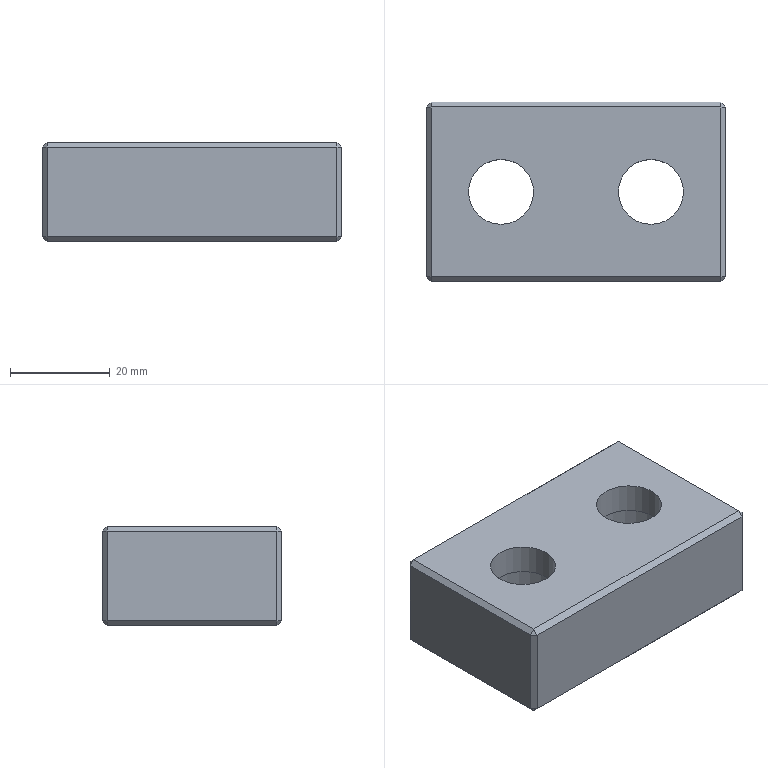Part | NX | features solid 2 | 1 solid | 32 faces | box 60 x 36 x 20 mm | volume 32584 mm3 | plane 28 | cylinder 4 | commonest cylinder face diameters 13 x2 20 x2
STEP:
#1=CARTESIAN_POINT('',(-28.,-137.,200.));
#2=VERTEX_POINT('',#1);
#3=CARTESIAN_POINT('',(30.,-137.,200.));
#4=VERTEX_POINT('',#3);
#5=CARTESIAN_POINT('',(-29.,-137.,200.));
#6=DIRECTION('',(-1.,0.,0.));
#7=VECTOR('',#6,1000.);
#8=LINE('',#5,#7);
#9=EDGE_CURVE('',#2,#4,#8,.F.);
#10=ORIENTED_EDGE('',*,*,#9,.F.);
#11=CARTESIAN_POINT('',(-28.,-171.,200.));
#12=VERTEX_POINT('',#11);
#13=CARTESIAN_POINT('',(-28.,-178.,200.));
#14=DIRECTION('',(0.,-1.,0.));
#15=VECTOR('',#14,1000.);
#16=LINE('',#13,#15);
#17=EDGE_CURVE('',#12,#2,#16,.F.);
#18=ORIENTED_EDGE('',*,*,#17,.F.);
#19=CARTESIAN_POINT('',(30.,-171.,200.));
#20=VERTEX_POINT('',#19);
#21=CARTESIAN_POINT('',(-29.,-171.,200.));
#22=DIRECTION('',(1.,0.,0.));
#23=VECTOR('',#22,1000.);
#24=LINE('',#21,#23);
#25=EDGE_CURVE('',#20,#12,#24,.F.);
#26=ORIENTED_EDGE('',*,*,#25,.F.);
#27=CARTESIAN_POINT('',(30.,-178.,200.));
#28=DIRECTION('',(0.,1.,0.));
#29=VECTOR('',#28,1000.);
#30=LINE('',#27,#29);
#31=EDGE_CURVE('',#4,#20,#30,.F.);
#32=ORIENTED_EDGE('',*,*,#31,.F.);
#33=EDGE_LOOP('',(#10,#18,#26,#32));
#34=FACE_BOUND('',#33,.T.);
#35=CARTESIAN_POINT('',(-14.,-147.5,200.));
#36=VERTEX_POINT('',#35);
#37=CARTESIAN_POINT('',(-14.,-154.,200.));
#38=DIRECTION('',(0.,0.,1.));
#39=DIRECTION('',(0.,1.,0.));
#40=AXIS2_PLACEMENT_3D('',#37,#38,#39);
#41=CIRCLE('',#40,6.5);
#42=EDGE_CURVE('',#36,#36,#41,.T.);
#43=ORIENTED_EDGE('',*,*,#42,.F.);
#44=EDGE_LOOP('',(#43));
#45=FACE_BOUND('',#44,.T.);
#46=CARTESIAN_POINT('',(16.,-147.5,200.));
#47=VERTEX_POINT('',#46);
#48=CARTESIAN_POINT('',(16.,-154.,200.));
#49=DIRECTION('',(0.,0.,1.));
#50=DIRECTION('',(0.,1.,0.));
#51=AXIS2_PLACEMENT_3D('',#48,#49,#50);
#52=CIRCLE('',#51,6.5);
#53=EDGE_CURVE('',#47,#47,#52,.T.);
#54=ORIENTED_EDGE('',*,*,#53,.F.);
#55=EDGE_LOOP('',(#54));
#56=FACE_BOUND('',#55,.T.);
#57=CARTESIAN_POINT('',(-29.,-178.,200.));
#58=DIRECTION('',(0.,0.,-1.));
#59=DIRECTION('',(1.,0.,0.));
#60=AXIS2_PLACEMENT_3D('',#57,#58,#59);
#61=PLANE('',#60);
#62=ADVANCED_FACE('',(#34,#45,#56),#61,.F.);
#63=CARTESIAN_POINT('',(16.,-144.,194.));
#64=VERTEX_POINT('',#63);
#65=CARTESIAN_POINT('',(16.,-154.,194.));
#66=DIRECTION('',(0.,0.,1.));
#67=DIRECTION('',(0.,1.,0.));
#68=AXIS2_PLACEMENT_3D('',#65,#66,#67);
#69=CIRCLE('',#68,10.);
#70=EDGE_CURVE('',#64,#64,#69,.T.);
#71=ORIENTED_EDGE('',*,*,#70,.F.);
#72=EDGE_LOOP('',(#71));
#73=FACE_BOUND('',#72,.T.);
#74=CARTESIAN_POINT('',(16.,-147.5,194.));
#75=VERTEX_POINT('',#74);
#76=CARTESIAN_POINT('',(16.,-154.,194.));
#77=DIRECTION('',(0.,0.,1.));
#78=DIRECTION('',(0.,1.,0.));
#79=AXIS2_PLACEMENT_3D('',#76,#77,#78);
#80=CIRCLE('',#79,6.5);
#81=EDGE_CURVE('',#75,#75,#80,.F.);
#82=ORIENTED_EDGE('',*,*,#81,.F.);
#83=EDGE_LOOP('',(#82));
#84=FACE_BOUND('',#83,.T.);
#85=CARTESIAN_POINT('',(16.,-154.,194.));
#86=DIRECTION('',(0.,0.,-1.));
#87=DIRECTION('',(0.,1.,0.));
#88=AXIS2_PLACEMENT_3D('',#85,#86,#87);
#89=PLANE('',#88);
#90=ADVANCED_FACE('',(#73,#84),#89,.T.);
#91=CARTESIAN_POINT('',(-14.,-144.,194.));
#92=VERTEX_POINT('',#91);
#93=CARTESIAN_POINT('',(-14.,-154.,194.));
#94=DIRECTION('',(0.,0.,1.));
#95=DIRECTION('',(0.,1.,0.));
#96=AXIS2_PLACEMENT_3D('',#93,#94,#95);
#97=CIRCLE('',#96,10.);
#98=EDGE_CURVE('',#92,#92,#97,.T.);
#99=ORIENTED_EDGE('',*,*,#98,.F.);
#100=EDGE_LOOP('',(#99));
#101=FACE_BOUND('',#100,.T.);
#102=CARTESIAN_POINT('',(-14.,-147.5,194.));
#103=VERTEX_POINT('',#102);
#104=CARTESIAN_POINT('',(-14.,-154.,194.));
#105=DIRECTION('',(0.,0.,1.));
#106=DIRECTION('',(0.,1.,0.));
#107=AXIS2_PLACEMENT_3D('',#104,#105,#106);
#108=CIRCLE('',#107,6.5);
#109=EDGE_CURVE('',#103,#103,#108,.F.);
#110=ORIENTED_EDGE('',*,*,#109,.F.);
#111=EDGE_LOOP('',(#110));
#112=FACE_BOUND('',#111,.T.);
#113=CARTESIAN_POINT('',(-14.,-154.,194.));
#114=DIRECTION('',(0.,0.,-1.));
#115=DIRECTION('',(0.,1.,0.));
#116=AXIS2_PLACEMENT_3D('',#113,#114,#115);
#117=PLANE('',#116);
#118=ADVANCED_FACE('',(#101,#112),#117,.T.);
#119=CARTESIAN_POINT('',(-28.,-171.,180.));
#120=VERTEX_POINT('',#119);
#121=CARTESIAN_POINT('',(30.,-171.,180.));
#122=VERTEX_POINT('',#121);
#123=CARTESIAN_POINT('',(31.,-171.,180.));
#124=DIRECTION('',(1.,0.,0.));
#125=VECTOR('',#124,1000.);
#126=LINE('',#123,#125);
#127=EDGE_CURVE('',#120,#122,#126,.T.);
#128=ORIENTED_EDGE('',*,*,#127,.F.);
#129=CARTESIAN_POINT('',(-28.,-137.,180.));
#130=VERTEX_POINT('',#129);
#131=CARTESIAN_POINT('',(-28.,-178.,180.));
#132=DIRECTION('',(0.,-1.,0.));
#133=VECTOR('',#132,1000.);
#134=LINE('',#131,#133);
#135=EDGE_CURVE('',#130,#120,#134,.T.);
#136=ORIENTED_EDGE('',*,*,#135,.F.);
#137=CARTESIAN_POINT('',(30.,-137.,180.));
#138=VERTEX_POINT('',#137);
#139=CARTESIAN_POINT('',(-29.,-137.,180.));
#140=DIRECTION('',(-1.,0.,0.));
#141=VECTOR('',#140,1000.);
#142=LINE('',#139,#141);
#143=EDGE_CURVE('',#138,#130,#142,.T.);
#144=ORIENTED_EDGE('',*,*,#143,.F.);
#145=CARTESIAN_POINT('',(30.,-178.,180.));
#146=DIRECTION('',(0.,1.,0.));
#147=VECTOR('',#146,1000.);
#148=LINE('',#145,#147);
#149=EDGE_CURVE('',#122,#138,#148,.T.);
#150=ORIENTED_EDGE('',*,*,#149,.F.);
#151=EDGE_LOOP('',(#128,#136,#144,#150));
#152=FACE_BOUND('',#151,.T.);
#153=CARTESIAN_POINT('',(-14.,-144.,180.));
#154=VERTEX_POINT('',#153);
#155=CARTESIAN_POINT('',(-14.,-154.,180.));
#156=DIRECTION('',(0.,0.,1.));
#157=DIRECTION('',(0.,1.,0.));
#158=AXIS2_PLACEMENT_3D('',#155,#156,#157);
#159=CIRCLE('',#158,10.);
#160=EDGE_CURVE('',#154,#154,#159,.T.);
#161=ORIENTED_EDGE('',*,*,#160,.T.);
#162=EDGE_LOOP('',(#161));
#163=FACE_BOUND('',#162,.T.);
#164=CARTESIAN_POINT('',(16.,-144.,180.));
#165=VERTEX_POINT('',#164);
#166=CARTESIAN_POINT('',(16.,-154.,180.));
#167=DIRECTION('',(0.,0.,1.));
#168=DIRECTION('',(0.,1.,0.));
#169=AXIS2_PLACEMENT_3D('',#166,#167,#168);
#170=CIRCLE('',#169,10.);
#171=EDGE_CURVE('',#165,#165,#170,.T.);
#172=ORIENTED_EDGE('',*,*,#171,.T.);
#173=EDGE_LOOP('',(#172));
#174=FACE_BOUND('',#173,.T.);
#175=CARTESIAN_POINT('',(-29.,-178.,180.));
#176=DIRECTION('',(0.,0.,-1.));
#177=DIRECTION('',(1.,0.,0.));
#178=AXIS2_PLACEMENT_3D('',#175,#176,#177);
#179=PLANE('',#178);
#180=ADVANCED_FACE('',(#152,#163,#174),#179,.T.);
#181=CARTESIAN_POINT('',(-29.,-171.,181.));
#182=VERTEX_POINT('',#181);
#183=CARTESIAN_POINT('',(-29.,-137.,181.));
#184=VERTEX_POINT('',#183);
#185=CARTESIAN_POINT('',(-29.,-178.,181.));
#186=DIRECTION('',(0.,-1.,0.));
#187=VECTOR('',#186,1000.);
#188=LINE('',#185,#187);
#189=EDGE_CURVE('',#182,#184,#188,.F.);
#190=ORIENTED_EDGE('',*,*,#189,.F.);
#191=CARTESIAN_POINT('',(-29.,-171.,199.));
#192=VERTEX_POINT('',#191);
#193=CARTESIAN_POINT('',(-29.,-171.,180.));
#194=DIRECTION('',(0.,0.,1.));
#195=VECTOR('',#194,1000.);
#196=LINE('',#193,#195);
#197=EDGE_CURVE('',#192,#182,#196,.F.);
#198=ORIENTED_EDGE('',*,*,#197,.F.);
#199=CARTESIAN_POINT('',(-29.,-137.,199.));
#200=VERTEX_POINT('',#199);
#201=CARTESIAN_POINT('',(-29.,-178.,199.));
#202=DIRECTION('',(0.,1.,0.));
#203=VECTOR('',#202,1000.);
#204=LINE('',#201,#203);
#205=EDGE_CURVE('',#200,#192,#204,.F.);
#206=ORIENTED_EDGE('',*,*,#205,.F.);
#207=CARTESIAN_POINT('',(-29.,-137.,180.));
#208=DIRECTION('',(0.,0.,-1.));
#209=VECTOR('',#208,1000.);
#210=LINE('',#207,#209);
#211=EDGE_CURVE('',#184,#200,#210,.F.);
#212=ORIENTED_EDGE('',*,*,#211,.F.);
#213=EDGE_LOOP('',(#190,#198,#206,#212));
#214=FACE_BOUND('',#213,.T.);
#215=CARTESIAN_POINT('',(-29.,-178.,180.));
#216=DIRECTION('',(1.,0.,0.));
#217=DIRECTION('',(0.,0.,1.));
#218=AXIS2_PLACEMENT_3D('',#215,#216,#217);
#219=PLANE('',#218);
#220=ADVANCED_FACE('',(#214),#219,.F.);
#221=CARTESIAN_POINT('',(31.,-171.,181.));
#222=VERTEX_POINT('',#221);
#223=CARTESIAN_POINT('',(31.,-171.,199.));
#224=VERTEX_POINT('',#223);
#225=CARTESIAN_POINT('',(31.,-171.,200.));
#226=DIRECTION('',(0.,0.,1.));
#227=VECTOR('',#226,1000.);
#228=LINE('',#225,#227);
#229=EDGE_CURVE('',#222,#224,#228,.T.);
#230=ORIENTED_EDGE('',*,*,#229,.F.);
#231=CARTESIAN_POINT('',(31.,-137.,181.));
#232=VERTEX_POINT('',#231);
#233=CARTESIAN_POINT('',(31.,-178.,181.));
#234=DIRECTION('',(0.,-1.,0.));
#235=VECTOR('',#234,1000.);
#236=LINE('',#233,#235);
#237=EDGE_CURVE('',#232,#222,#236,.T.);
#238=ORIENTED_EDGE('',*,*,#237,.F.);
#239=CARTESIAN_POINT('',(31.,-137.,199.));
#240=VERTEX_POINT('',#239);
#241=CARTESIAN_POINT('',(31.,-137.,180.));
#242=DIRECTION('',(0.,0.,-1.));
#243=VECTOR('',#242,1000.);
#244=LINE('',#241,#243);
#245=EDGE_CURVE('',#240,#232,#244,.T.);
#246=ORIENTED_EDGE('',*,*,#245,.F.);
#247=CARTESIAN_POINT('',(31.,-178.,199.));
#248=DIRECTION('',(0.,1.,0.));
#249=VECTOR('',#248,1000.);
#250=LINE('',#247,#249);
#251=EDGE_CURVE('',#224,#240,#250,.T.);
#252=ORIENTED_EDGE('',*,*,#251,.F.);
#253=EDGE_LOOP('',(#230,#238,#246,#252));
#254=FACE_BOUND('',#253,.T.);
#255=CARTESIAN_POINT('',(31.,-178.,180.));
#256=DIRECTION('',(1.,0.,0.));
#257=DIRECTION('',(0.,0.,1.));
#258=AXIS2_PLACEMENT_3D('',#255,#256,#257);
#259=PLANE('',#258);
#260=ADVANCED_FACE('',(#254),#259,.T.);
#261=CARTESIAN_POINT('',(30.,-172.,181.));
#262=VERTEX_POINT('',#261);
#263=CARTESIAN_POINT('',(-28.,-172.,181.));
#264=VERTEX_POINT('',#263);
#265=CARTESIAN_POINT('',(-29.,-172.,181.));
#266=DIRECTION('',(-1.,0.,0.));
#267=VECTOR('',#266,1000.);
#268=LINE('',#265,#267);
#269=EDGE_CURVE('',#262,#264,#268,.T.);
#270=ORIENTED_EDGE('',*,*,#269,.F.);
#271=CARTESIAN_POINT('',(30.,-172.,199.));
#272=VERTEX_POINT('',#271);
#273=CARTESIAN_POINT('',(30.,-172.,180.));
#274=DIRECTION('',(0.,0.,-1.));
#275=VECTOR('',#274,1000.);
#276=LINE('',#273,#275);
#277=EDGE_CURVE('',#272,#262,#276,.T.);
#278=ORIENTED_EDGE('',*,*,#277,.F.);
#279=CARTESIAN_POINT('',(-28.,-172.,199.));
#280=VERTEX_POINT('',#279);
#281=CARTESIAN_POINT('',(31.,-172.,199.));
#282=DIRECTION('',(1.,0.,0.));
#283=VECTOR('',#282,1000.);
#284=LINE('',#281,#283);
#285=EDGE_CURVE('',#280,#272,#284,.T.);
#286=ORIENTED_EDGE('',*,*,#285,.F.);
#287=CARTESIAN_POINT('',(-28.,-172.,200.));
#288=DIRECTION('',(0.,0.,1.));
#289=VECTOR('',#288,1000.);
#290=LINE('',#287,#289);
#291=EDGE_CURVE('',#264,#280,#290,.T.);
#292=ORIENTED_EDGE('',*,*,#291,.F.);
#293=EDGE_LOOP('',(#270,#278,#286,#292));
#294=FACE_BOUND('',#293,.T.);
#295=CARTESIAN_POINT('',(-29.,-172.,180.));
#296=DIRECTION('',(0.,1.,0.));
#297=DIRECTION('',(0.,0.,1.));
#298=AXIS2_PLACEMENT_3D('',#295,#296,#297);
#299=PLANE('',#298);
#300=ADVANCED_FACE('',(#294),#299,.F.);
#301=CARTESIAN_POINT('',(-28.,-136.,181.));
#302=VERTEX_POINT('',#301);
#303=CARTESIAN_POINT('',(30.,-136.,181.));
#304=VERTEX_POINT('',#303);
#305=CARTESIAN_POINT('',(-29.,-136.,181.));
#306=DIRECTION('',(1.,0.,0.));
#307=VECTOR('',#306,1000.);
#308=LINE('',#305,#307);
#309=EDGE_CURVE('',#302,#304,#308,.T.);
#310=ORIENTED_EDGE('',*,*,#309,.F.);
#311=CARTESIAN_POINT('',(-28.,-136.,199.));
#312=VERTEX_POINT('',#311);
#313=CARTESIAN_POINT('',(-28.,-136.,180.));
#314=DIRECTION('',(0.,0.,-1.));
#315=VECTOR('',#314,1000.);
#316=LINE('',#313,#315);
#317=EDGE_CURVE('',#312,#302,#316,.T.);
#318=ORIENTED_EDGE('',*,*,#317,.F.);
#319=CARTESIAN_POINT('',(30.,-136.,199.));
#320=VERTEX_POINT('',#319);
#321=CARTESIAN_POINT('',(-29.,-136.,199.));
#322=DIRECTION('',(-1.,0.,0.));
#323=VECTOR('',#322,1000.);
#324=LINE('',#321,#323);
#325=EDGE_CURVE('',#320,#312,#324,.T.);
#326=ORIENTED_EDGE('',*,*,#325,.F.);
#327=CARTESIAN_POINT('',(30.,-136.,180.));
#328=DIRECTION('',(0.,0.,1.));
#329=VECTOR('',#328,1000.);
#330=LINE('',#327,#329);
#331=EDGE_CURVE('',#304,#320,#330,.T.);
#332=ORIENTED_EDGE('',*,*,#331,.F.);
#333=EDGE_LOOP('',(#310,#318,#326,#332));
#334=FACE_BOUND('',#333,.T.);
#335=CARTESIAN_POINT('',(-29.,-136.,180.));
#336=DIRECTION('',(0.,1.,0.));
#337=DIRECTION('',(0.,0.,1.));
#338=AXIS2_PLACEMENT_3D('',#335,#336,#337);
#339=PLANE('',#338);
#340=ADVANCED_FACE('',(#334),#339,.T.);
#341=ORIENTED_EDGE('',*,*,#160,.F.);
#342=EDGE_LOOP('',(#341));
#343=FACE_BOUND('',#342,.T.);
#344=ORIENTED_EDGE('',*,*,#98,.T.);
#345=EDGE_LOOP('',(#344));
#346=FACE_BOUND('',#345,.T.);
#347=CARTESIAN_POINT('',(-14.,-154.,180.));
#348=DIRECTION('',(0.,0.,1.));
#349=DIRECTION('',(0.,-1.,0.));
#350=AXIS2_PLACEMENT_3D('',#347,#348,#349);
#351=CYLINDRICAL_SURFACE('',#350,10.);
#352=ADVANCED_FACE('',(#343,#346),#351,.F.);
#353=ORIENTED_EDGE('',*,*,#171,.F.);
#354=EDGE_LOOP('',(#353));
#355=FACE_BOUND('',#354,.T.);
#356=ORIENTED_EDGE('',*,*,#70,.T.);
#357=EDGE_LOOP('',(#356));
#358=FACE_BOUND('',#357,.T.);
#359=CARTESIAN_POINT('',(16.,-154.,180.));
#360=DIRECTION('',(0.,0.,1.));
#361=DIRECTION('',(0.,-1.,0.));
#362=AXIS2_PLACEMENT_3D('',#359,#360,#361);
#363=CYLINDRICAL_SURFACE('',#362,10.);
#364=ADVANCED_FACE('',(#355,#358),#363,.F.);
#365=ORIENTED_EDGE('',*,*,#42,.T.);
#366=EDGE_LOOP('',(#365));
#367=FACE_BOUND('',#366,.T.);
#368=ORIENTED_EDGE('',*,*,#109,.T.);
#369=EDGE_LOOP('',(#368));
#370=FACE_BOUND('',#369,.T.);
#371=CARTESIAN_POINT('',(-14.,-154.,180.));
#372=DIRECTION('',(0.,0.,1.));
#373=DIRECTION('',(0.,-1.,0.));
#374=AXIS2_PLACEMENT_3D('',#371,#372,#373);
#375=CYLINDRICAL_SURFACE('',#374,6.5);
#376=ADVANCED_FACE('',(#367,#370),#375,.F.);
#377=ORIENTED_EDGE('',*,*,#53,.T.);
#378=EDGE_LOOP('',(#377));
#379=FACE_BOUND('',#378,.T.);
#380=ORIENTED_EDGE('',*,*,#81,.T.);
#381=EDGE_LOOP('',(#380));
#382=FACE_BOUND('',#381,.T.);
#383=CARTESIAN_POINT('',(16.,-154.,180.));
#384=DIRECTION('',(0.,0.,1.));
#385=DIRECTION('',(0.,-1.,0.));
#386=AXIS2_PLACEMENT_3D('',#383,#384,#385);
#387=CYLINDRICAL_SURFACE('',#386,6.5);
#388=ADVANCED_FACE('',(#379,#382),#387,.F.);
#389=CARTESIAN_POINT('',(-28.5,-137.,180.5));
#390=DIRECTION('',(0.7071,0.,-0.7071));
#391=VECTOR('',#390,1000.);
#392=LINE('',#389,#391);
#393=EDGE_CURVE('',#184,#130,#392,.T.);
#394=ORIENTED_EDGE('',*,*,#393,.T.);
#395=ORIENTED_EDGE('',*,*,#135,.T.);
#396=CARTESIAN_POINT('',(-29.,-171.,181.));
#397=DIRECTION('',(-0.7071,0.,0.7071));
#398=VECTOR('',#397,1000.);
#399=LINE('',#396,#398);
#400=EDGE_CURVE('',#120,#182,#399,.T.);
#401=ORIENTED_EDGE('',*,*,#400,.T.);
#402=ORIENTED_EDGE('',*,*,#189,.T.);
#403=EDGE_LOOP('',(#394,#395,#401,#402));
#404=FACE_BOUND('',#403,.T.);
#405=CARTESIAN_POINT('',(-28.,-178.,180.));
#406=DIRECTION('',(-0.7071,0.,-0.7071));
#407=DIRECTION('',(0.7071,0.,-0.7071));
#408=AXIS2_PLACEMENT_3D('',#405,#406,#407);
#409=PLANE('',#408);
#410=ADVANCED_FACE('',(#404),#409,.T.);
#411=CARTESIAN_POINT('',(-28.,-136.,181.));
#412=DIRECTION('',(-0.7071,-0.7071,0.));
#413=VECTOR('',#412,1000.);
#414=LINE('',#411,#413);
#415=EDGE_CURVE('',#184,#302,#414,.F.);
#416=ORIENTED_EDGE('',*,*,#415,.T.);
#417=CARTESIAN_POINT('',(-28.,-136.,181.));
#418=DIRECTION('',(0.,-0.7071,-0.7071));
#419=VECTOR('',#418,1000.);
#420=LINE('',#417,#419);
#421=EDGE_CURVE('',#302,#130,#420,.T.);
#422=ORIENTED_EDGE('',*,*,#421,.T.);
#423=ORIENTED_EDGE('',*,*,#393,.F.);
#424=EDGE_LOOP('',(#416,#422,#423));
#425=FACE_BOUND('',#424,.T.);
#426=CARTESIAN_POINT('',(-28.,-136.,181.));
#427=DIRECTION('',(-0.5774,0.5774,-0.5774));
#428=DIRECTION('',(0.,0.7071,0.7071));
#429=AXIS2_PLACEMENT_3D('',#426,#427,#428);
#430=PLANE('',#429);
#431=ADVANCED_FACE('',(#425),#430,.T.);
#432=CARTESIAN_POINT('',(-28.,-171.5,180.5));
#433=DIRECTION('',(0.,0.7071,-0.7071));
#434=VECTOR('',#433,1000.);
#435=LINE('',#432,#434);
#436=EDGE_CURVE('',#120,#264,#435,.F.);
#437=ORIENTED_EDGE('',*,*,#436,.T.);
#438=CARTESIAN_POINT('',(-29.,-171.,181.));
#439=DIRECTION('',(-0.7071,0.7071,0.));
#440=VECTOR('',#439,1000.);
#441=LINE('',#438,#440);
#442=EDGE_CURVE('',#264,#182,#441,.T.);
#443=ORIENTED_EDGE('',*,*,#442,.T.);
#444=ORIENTED_EDGE('',*,*,#400,.F.);
#445=EDGE_LOOP('',(#437,#443,#444));
#446=FACE_BOUND('',#445,.T.);
#447=CARTESIAN_POINT('',(-29.,-171.,181.));
#448=DIRECTION('',(-0.5774,-0.5774,-0.5774));
#449=DIRECTION('',(0.,0.7071,-0.7071));
#450=AXIS2_PLACEMENT_3D('',#447,#448,#449);
#451=PLANE('',#450);
#452=ADVANCED_FACE('',(#446),#451,.T.);
#453=ORIENTED_EDGE('',*,*,#421,.F.);
#454=ORIENTED_EDGE('',*,*,#309,.T.);
#455=CARTESIAN_POINT('',(30.,-136.5,180.5));
#456=DIRECTION('',(0.,0.7071,0.7071));
#457=VECTOR('',#456,1000.);
#458=LINE('',#455,#457);
#459=EDGE_CURVE('',#304,#138,#458,.F.);
#460=ORIENTED_EDGE('',*,*,#459,.T.);
#461=ORIENTED_EDGE('',*,*,#143,.T.);
#462=EDGE_LOOP('',(#453,#454,#460,#461));
#463=FACE_BOUND('',#462,.T.);
#464=CARTESIAN_POINT('',(-29.,-136.,181.));
#465=DIRECTION('',(0.,-0.7071,0.7071));
#466=DIRECTION('',(0.,-0.7071,-0.7071));
#467=AXIS2_PLACEMENT_3D('',#464,#465,#466);
#468=PLANE('',#467);
#469=ADVANCED_FACE('',(#463),#468,.F.);
#470=ORIENTED_EDGE('',*,*,#415,.F.);
#471=ORIENTED_EDGE('',*,*,#211,.T.);
#472=CARTESIAN_POINT('',(-28.,-136.,199.));
#473=DIRECTION('',(0.7071,0.7071,0.));
#474=VECTOR('',#473,1000.);
#475=LINE('',#472,#474);
#476=EDGE_CURVE('',#200,#312,#475,.T.);
#477=ORIENTED_EDGE('',*,*,#476,.T.);
#478=ORIENTED_EDGE('',*,*,#317,.T.);
#479=EDGE_LOOP('',(#470,#471,#477,#478));
#480=FACE_BOUND('',#479,.T.);
#481=CARTESIAN_POINT('',(-29.,-137.,180.));
#482=DIRECTION('',(-0.7071,0.7071,0.));
#483=DIRECTION('',(-0.7071,-0.7071,0.));
#484=AXIS2_PLACEMENT_3D('',#481,#482,#483);
#485=PLANE('',#484);
#486=ADVANCED_FACE('',(#480),#485,.T.);
#487=CARTESIAN_POINT('',(-29.,-171.,199.));
#488=DIRECTION('',(-0.7071,0.,-0.7071));
#489=VECTOR('',#488,1000.);
#490=LINE('',#487,#489);
#491=EDGE_CURVE('',#192,#12,#490,.F.);
#492=ORIENTED_EDGE('',*,*,#491,.T.);
#493=ORIENTED_EDGE('',*,*,#17,.T.);
#494=CARTESIAN_POINT('',(-28.5,-137.,199.5));
#495=DIRECTION('',(0.7071,0.,0.7071));
#496=VECTOR('',#495,1000.);
#497=LINE('',#494,#496);
#498=EDGE_CURVE('',#2,#200,#497,.F.);
#499=ORIENTED_EDGE('',*,*,#498,.T.);
#500=ORIENTED_EDGE('',*,*,#205,.T.);
#501=EDGE_LOOP('',(#492,#493,#499,#500));
#502=FACE_BOUND('',#501,.T.);
#503=CARTESIAN_POINT('',(-29.,-178.,199.));
#504=DIRECTION('',(0.7071,0.,-0.7071));
#505=DIRECTION('',(0.7071,0.,0.7071));
#506=AXIS2_PLACEMENT_3D('',#503,#504,#505);
#507=PLANE('',#506);
#508=ADVANCED_FACE('',(#502),#507,.F.);
#509=ORIENTED_EDGE('',*,*,#442,.F.);
#510=ORIENTED_EDGE('',*,*,#291,.T.);
#511=CARTESIAN_POINT('',(-29.,-171.,199.));
#512=DIRECTION('',(0.7071,-0.7071,0.));
#513=VECTOR('',#512,1000.);
#514=LINE('',#511,#513);
#515=EDGE_CURVE('',#280,#192,#514,.F.);
#516=ORIENTED_EDGE('',*,*,#515,.T.);
#517=ORIENTED_EDGE('',*,*,#197,.T.);
#518=EDGE_LOOP('',(#509,#510,#516,#517));
#519=FACE_BOUND('',#518,.T.);
#520=CARTESIAN_POINT('',(-28.,-172.,180.));
#521=DIRECTION('',(0.7071,0.7071,0.));
#522=DIRECTION('',(-0.7071,0.7071,0.));
#523=AXIS2_PLACEMENT_3D('',#520,#521,#522);
#524=PLANE('',#523);
#525=ADVANCED_FACE('',(#519),#524,.F.);
#526=ORIENTED_EDGE('',*,*,#436,.F.);
#527=ORIENTED_EDGE('',*,*,#127,.T.);
#528=CARTESIAN_POINT('',(30.,-172.,181.));
#529=DIRECTION('',(0.,-0.7071,0.7071));
#530=VECTOR('',#529,1000.);
#531=LINE('',#528,#530);
#532=EDGE_CURVE('',#122,#262,#531,.T.);
#533=ORIENTED_EDGE('',*,*,#532,.T.);
#534=ORIENTED_EDGE('',*,*,#269,.T.);
#535=EDGE_LOOP('',(#526,#527,#533,#534));
#536=FACE_BOUND('',#535,.T.);
#537=CARTESIAN_POINT('',(-29.,-171.,180.));
#538=DIRECTION('',(0.,-0.7071,-0.7071));
#539=DIRECTION('',(0.,0.7071,-0.7071));
#540=AXIS2_PLACEMENT_3D('',#537,#538,#539);
#541=PLANE('',#540);
#542=ADVANCED_FACE('',(#536),#541,.T.);
#543=CARTESIAN_POINT('',(31.,-137.,181.));
#544=DIRECTION('',(-0.7071,0.,-0.7071));
#545=VECTOR('',#544,1000.);
#546=LINE('',#543,#545);
#547=EDGE_CURVE('',#138,#232,#546,.F.);
#548=ORIENTED_EDGE('',*,*,#547,.T.);
#549=ORIENTED_EDGE('',*,*,#237,.T.);
#550=CARTESIAN_POINT('',(30.5,-171.,180.5));
#551=DIRECTION('',(0.7071,0.,0.7071));
#552=VECTOR('',#551,1000.);
#553=LINE('',#550,#552);
#554=EDGE_CURVE('',#222,#122,#553,.F.);
#555=ORIENTED_EDGE('',*,*,#554,.T.);
#556=ORIENTED_EDGE('',*,*,#149,.T.);
#557=EDGE_LOOP('',(#548,#549,#555,#556));
#558=FACE_BOUND('',#557,.T.);
#559=CARTESIAN_POINT('',(31.,-178.,181.));
#560=DIRECTION('',(-0.7071,0.,0.7071));
#561=DIRECTION('',(-0.7071,0.,-0.7071));
#562=AXIS2_PLACEMENT_3D('',#559,#560,#561);
#563=PLANE('',#562);
#564=ADVANCED_FACE('',(#558),#563,.F.);
#565=ORIENTED_EDGE('',*,*,#459,.F.);
#566=CARTESIAN_POINT('',(31.,-137.,181.));
#567=DIRECTION('',(0.7071,-0.7071,0.));
#568=VECTOR('',#567,1000.);
#569=LINE('',#566,#568);
#570=EDGE_CURVE('',#304,#232,#569,.T.);
#571=ORIENTED_EDGE('',*,*,#570,.T.);
#572=ORIENTED_EDGE('',*,*,#547,.F.);
#573=EDGE_LOOP('',(#565,#571,#572));
#574=FACE_BOUND('',#573,.T.);
#575=CARTESIAN_POINT('',(31.,-137.,181.));
#576=DIRECTION('',(0.5774,0.5774,-0.5774));
#577=DIRECTION('',(0.,0.7071,0.7071));
#578=AXIS2_PLACEMENT_3D('',#575,#576,#577);
#579=PLANE('',#578);
#580=ADVANCED_FACE('',(#574),#579,.T.);
#581=ORIENTED_EDGE('',*,*,#498,.F.);
#582=CARTESIAN_POINT('',(-28.,-136.,199.));
#583=DIRECTION('',(0.,-0.7071,0.7071));
#584=VECTOR('',#583,1000.);
#585=LINE('',#582,#584);
#586=EDGE_CURVE('',#2,#312,#585,.F.);
#587=ORIENTED_EDGE('',*,*,#586,.T.);
#588=ORIENTED_EDGE('',*,*,#476,.F.);
#589=EDGE_LOOP('',(#581,#587,#588));
#590=FACE_BOUND('',#589,.T.);
#591=CARTESIAN_POINT('',(-28.,-136.,199.));
#592=DIRECTION('',(-0.5774,0.5774,0.5774));
#593=DIRECTION('',(0.,-0.7071,0.7071));
#594=AXIS2_PLACEMENT_3D('',#591,#592,#593);
#595=PLANE('',#594);
#596=ADVANCED_FACE('',(#590),#595,.T.);
#597=ORIENTED_EDGE('',*,*,#515,.F.);
#598=CARTESIAN_POINT('',(-28.,-171.5,199.5));
#599=DIRECTION('',(0.,0.7071,0.7071));
#600=VECTOR('',#599,1000.);
#601=LINE('',#598,#600);
#602=EDGE_CURVE('',#280,#12,#601,.T.);
#603=ORIENTED_EDGE('',*,*,#602,.T.);
#604=ORIENTED_EDGE('',*,*,#491,.F.);
#605=EDGE_LOOP('',(#597,#603,#604));
#606=FACE_BOUND('',#605,.T.);
#607=CARTESIAN_POINT('',(-29.,-171.,199.));
#608=DIRECTION('',(-0.5774,-0.5774,0.5774));
#609=DIRECTION('',(0.,-0.7071,-0.7071));
#610=AXIS2_PLACEMENT_3D('',#607,#608,#609);
#611=PLANE('',#610);
#612=ADVANCED_FACE('',(#606),#611,.T.);
#613=ORIENTED_EDGE('',*,*,#554,.F.);
#614=CARTESIAN_POINT('',(30.,-172.,181.));
#615=DIRECTION('',(0.7071,0.7071,0.));
#616=VECTOR('',#615,1000.);
#617=LINE('',#614,#616);
#618=EDGE_CURVE('',#222,#262,#617,.F.);
#619=ORIENTED_EDGE('',*,*,#618,.T.);
#620=ORIENTED_EDGE('',*,*,#532,.F.);
#621=EDGE_LOOP('',(#613,#619,#620));
#622=FACE_BOUND('',#621,.T.);
#623=CARTESIAN_POINT('',(30.,-172.,181.));
#624=DIRECTION('',(0.5774,-0.5774,-0.5774));
#625=DIRECTION('',(0.,0.7071,-0.7071));
#626=AXIS2_PLACEMENT_3D('',#623,#624,#625);
#627=PLANE('',#626);
#628=ADVANCED_FACE('',(#622),#627,.T.);
#629=ORIENTED_EDGE('',*,*,#570,.F.);
#630=ORIENTED_EDGE('',*,*,#331,.T.);
#631=CARTESIAN_POINT('',(31.,-137.,199.));
#632=DIRECTION('',(-0.7071,0.7071,0.));
#633=VECTOR('',#632,1000.);
#634=LINE('',#631,#633);
#635=EDGE_CURVE('',#320,#240,#634,.F.);
#636=ORIENTED_EDGE('',*,*,#635,.T.);
#637=ORIENTED_EDGE('',*,*,#245,.T.);
#638=EDGE_LOOP('',(#629,#630,#636,#637));
#639=FACE_BOUND('',#638,.T.);
#640=CARTESIAN_POINT('',(30.,-136.,180.));
#641=DIRECTION('',(-0.7071,-0.7071,0.));
#642=DIRECTION('',(0.7071,-0.7071,0.));
#643=AXIS2_PLACEMENT_3D('',#640,#641,#642);
#644=PLANE('',#643);
#645=ADVANCED_FACE('',(#639),#644,.F.);
#646=ORIENTED_EDGE('',*,*,#586,.F.);
#647=ORIENTED_EDGE('',*,*,#9,.T.);
#648=CARTESIAN_POINT('',(30.,-136.5,199.5));
#649=DIRECTION('',(0.,0.7071,-0.7071));
#650=VECTOR('',#649,1000.);
#651=LINE('',#648,#650);
#652=EDGE_CURVE('',#4,#320,#651,.T.);
#653=ORIENTED_EDGE('',*,*,#652,.T.);
#654=ORIENTED_EDGE('',*,*,#325,.T.);
#655=EDGE_LOOP('',(#646,#647,#653,#654));
#656=FACE_BOUND('',#655,.T.);
#657=CARTESIAN_POINT('',(-29.,-137.,200.));
#658=DIRECTION('',(0.,0.7071,0.7071));
#659=DIRECTION('',(0.,-0.7071,0.7071));
#660=AXIS2_PLACEMENT_3D('',#657,#658,#659);
#661=PLANE('',#660);
#662=ADVANCED_FACE('',(#656),#661,.T.);
#663=ORIENTED_EDGE('',*,*,#602,.F.);
#664=ORIENTED_EDGE('',*,*,#285,.T.);
#665=CARTESIAN_POINT('',(30.,-171.,200.));
#666=DIRECTION('',(0.,-0.7071,-0.7071));
#667=VECTOR('',#666,1000.);
#668=LINE('',#665,#667);
#669=EDGE_CURVE('',#272,#20,#668,.F.);
#670=ORIENTED_EDGE('',*,*,#669,.T.);
#671=ORIENTED_EDGE('',*,*,#25,.T.);
#672=EDGE_LOOP('',(#663,#664,#670,#671));
#673=FACE_BOUND('',#672,.T.);
#674=CARTESIAN_POINT('',(-29.,-172.,199.));
#675=DIRECTION('',(0.,0.7071,-0.7071));
#676=DIRECTION('',(0.,0.7071,0.7071));
#677=AXIS2_PLACEMENT_3D('',#674,#675,#676);
#678=PLANE('',#677);
#679=ADVANCED_FACE('',(#673),#678,.F.);
#680=ORIENTED_EDGE('',*,*,#618,.F.);
#681=ORIENTED_EDGE('',*,*,#229,.T.);
#682=CARTESIAN_POINT('',(30.5,-171.5,199.));
#683=DIRECTION('',(-0.7071,-0.7071,0.));
#684=VECTOR('',#683,1000.);
#685=LINE('',#682,#684);
#686=EDGE_CURVE('',#224,#272,#685,.T.);
#687=ORIENTED_EDGE('',*,*,#686,.T.);
#688=ORIENTED_EDGE('',*,*,#277,.T.);
#689=EDGE_LOOP('',(#680,#681,#687,#688));
#690=FACE_BOUND('',#689,.T.);
#691=CARTESIAN_POINT('',(31.,-171.,180.));
#692=DIRECTION('',(0.7071,-0.7071,0.));
#693=DIRECTION('',(0.7071,0.7071,0.));
#694=AXIS2_PLACEMENT_3D('',#691,#692,#693);
#695=PLANE('',#694);
#696=ADVANCED_FACE('',(#690),#695,.T.);
#697=ORIENTED_EDGE('',*,*,#652,.F.);
#698=CARTESIAN_POINT('',(31.,-137.,199.));
#699=DIRECTION('',(-0.7071,0.,0.7071));
#700=VECTOR('',#699,1000.);
#701=LINE('',#698,#700);
#702=EDGE_CURVE('',#4,#240,#701,.F.);
#703=ORIENTED_EDGE('',*,*,#702,.T.);
#704=ORIENTED_EDGE('',*,*,#635,.F.);
#705=EDGE_LOOP('',(#697,#703,#704));
#706=FACE_BOUND('',#705,.T.);
#707=CARTESIAN_POINT('',(31.,-137.,199.));
#708=DIRECTION('',(0.5774,0.5774,0.5774));
#709=DIRECTION('',(0.,-0.7071,0.7071));
#710=AXIS2_PLACEMENT_3D('',#707,#708,#709);
#711=PLANE('',#710);
#712=ADVANCED_FACE('',(#706),#711,.T.);
#713=ORIENTED_EDGE('',*,*,#686,.F.);
#714=CARTESIAN_POINT('',(30.,-171.,200.));
#715=DIRECTION('',(0.7071,0.,-0.7071));
#716=VECTOR('',#715,1000.);
#717=LINE('',#714,#716);
#718=EDGE_CURVE('',#224,#20,#717,.F.);
#719=ORIENTED_EDGE('',*,*,#718,.T.);
#720=ORIENTED_EDGE('',*,*,#669,.F.);
#721=EDGE_LOOP('',(#713,#719,#720));
#722=FACE_BOUND('',#721,.T.);
#723=CARTESIAN_POINT('',(30.,-171.,200.));
#724=DIRECTION('',(0.5774,-0.5774,0.5774));
#725=DIRECTION('',(0.,-0.7071,-0.7071));
#726=AXIS2_PLACEMENT_3D('',#723,#724,#725);
#727=PLANE('',#726);
#728=ADVANCED_FACE('',(#722),#727,.T.);
#729=ORIENTED_EDGE('',*,*,#702,.F.);
#730=ORIENTED_EDGE('',*,*,#31,.T.);
#731=ORIENTED_EDGE('',*,*,#718,.F.);
#732=ORIENTED_EDGE('',*,*,#251,.T.);
#733=EDGE_LOOP('',(#729,#730,#731,#732));
#734=FACE_BOUND('',#733,.T.);
#735=CARTESIAN_POINT('',(30.,-178.,200.));
#736=DIRECTION('',(0.7071,0.,0.7071));
#737=DIRECTION('',(-0.7071,0.,0.7071));
#738=AXIS2_PLACEMENT_3D('',#735,#736,#737);
#739=PLANE('',#738);
#740=ADVANCED_FACE('',(#734),#739,.T.);
#741=CLOSED_SHELL('',(#62,#90,#118,#180,#220,#260,#300,#340,#352,#364,#376,#388,#410,#431,#452,#469,#486,#508,#525,#542,#564,#580,#596,#612,#628,#645,#662,#679,#696,#712,#728,#740));
#742=MANIFOLD_SOLID_BREP('',#741);
#743=(LENGTH_UNIT()NAMED_UNIT(*)SI_UNIT(.MILLI.,.METRE.));
#744=UNCERTAINTY_MEASURE_WITH_UNIT(LENGTH_MEASURE(0.00001),#743,'','');
#745=(NAMED_UNIT(*)PLANE_ANGLE_UNIT()SI_UNIT($,.RADIAN.));
#746=(NAMED_UNIT(*)SI_UNIT($,.STERADIAN.)SOLID_ANGLE_UNIT());
#747=(GEOMETRIC_REPRESENTATION_CONTEXT(3)GLOBAL_UNCERTAINTY_ASSIGNED_CONTEXT((#744))GLOBAL_UNIT_ASSIGNED_CONTEXT((#743,#745,#746))REPRESENTATION_CONTEXT('',''));
#748=ADVANCED_BREP_SHAPE_REPRESENTATION('',(#742),#747);